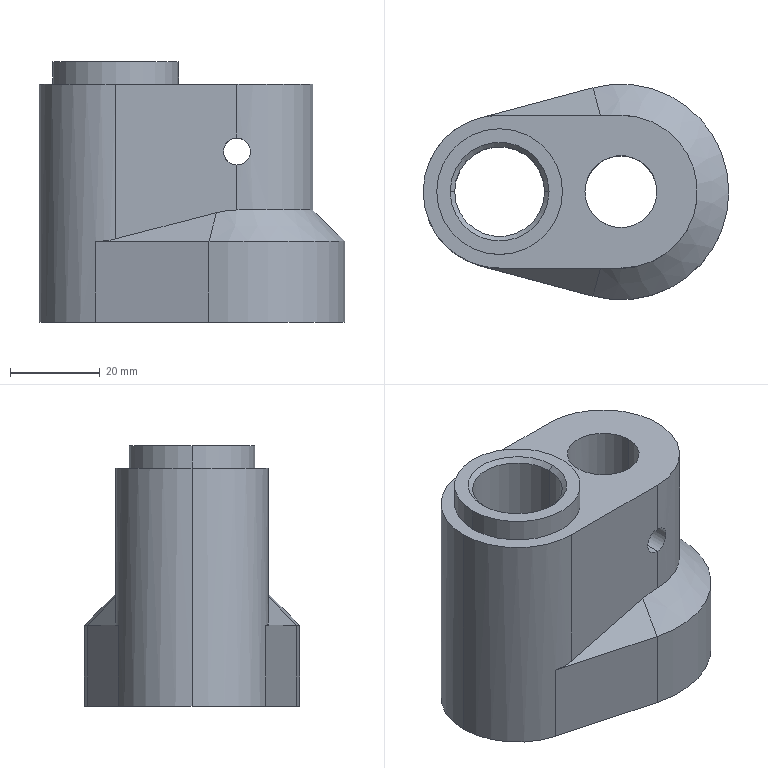Part | SolidWorks | features ICE 7, Chamfer 2, Extrusion 1, HoleWzd 1 | 1 solid | 52 faces | box 68 x 48 x 58 mm | volume 60377 mm3 | cylinder 23 | cone 19 | plane 10 | commonest cylinder face diameters 2.5 x6 6 x4 34 x3 16 x2 20 x2 28 x2